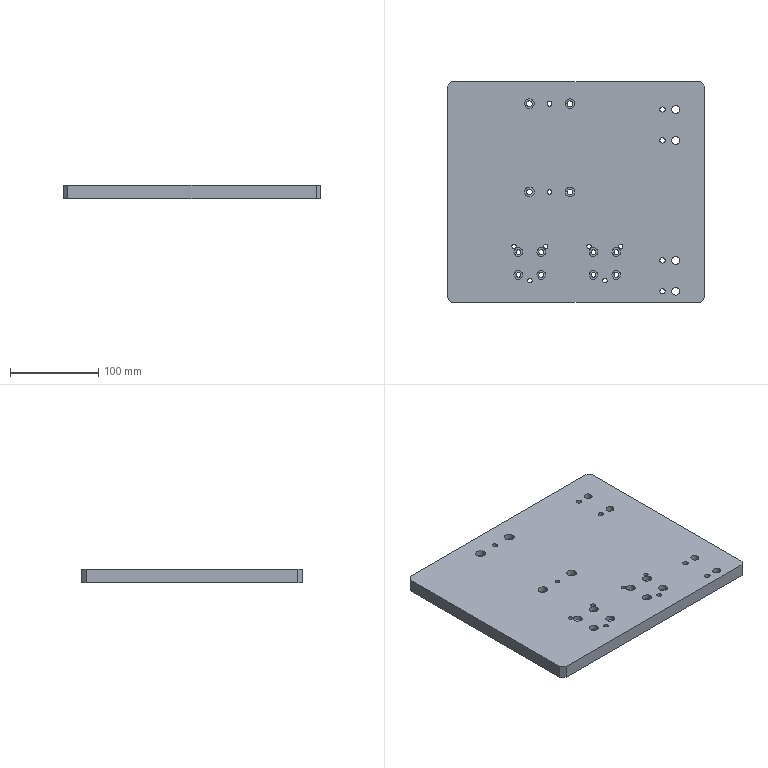Part | 1 solid | 136 faces | box 292 x 250 x 15 mm | volume 1072979 mm3 | cylinder 98 | plane 28 | cone 10 | commonest cylinder face diameters 5 x16 5.5 x16 10 x16 6 x8 6.6 x8 9 x8